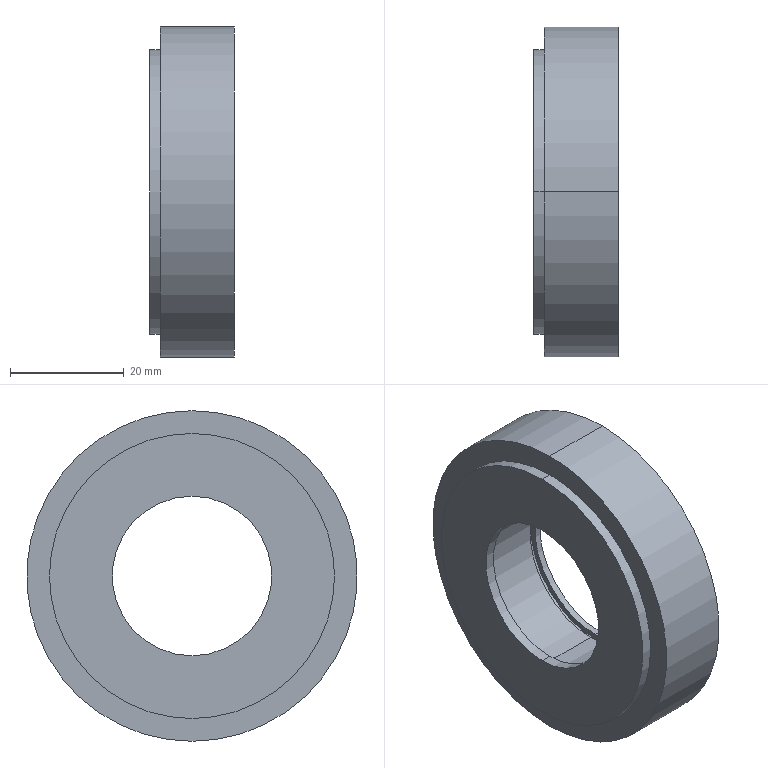Part | SolidWorks | features Revolution 1 | 1 solid | 21 faces | box 14.9 x 58 x 58 mm | volume 27501 mm3 | cylinder 14 | plane 7 | commonest cylinder face diameters 30 x4 28 x2 32 x2 34 x2 50 x2 58 x2
STEP:
#1=CARTESIAN_POINT('',(1.9,0.,25.));
#2=VERTEX_POINT('',#1);
#3=CARTESIAN_POINT('',(1.9,0.,-25.));
#4=VERTEX_POINT('',#3);
#5=CARTESIAN_POINT('',(1.9,0.,0.));
#6=DIRECTION('',(-1.,0.,0.));
#7=DIRECTION('',(0.,0.,1.));
#8=AXIS2_PLACEMENT_3D('',#5,#6,#7);
#9=CIRCLE('',#8,25.);
#10=EDGE_CURVE('',#2,#4,#9,.T.);
#11=ORIENTED_EDGE('',*,*,#10,.T.);
#12=CARTESIAN_POINT('',(0.,0.,-25.));
#13=VERTEX_POINT('',#12);
#14=CARTESIAN_POINT('',(-10.496,0.,-25.));
#15=DIRECTION('',(-1.,0.,0.));
#16=VECTOR('',#15,1000.);
#17=LINE('',#14,#16);
#18=EDGE_CURVE('',#4,#13,#17,.T.);
#19=ORIENTED_EDGE('',*,*,#18,.T.);
#20=CARTESIAN_POINT('',(0.,0.,25.));
#21=VERTEX_POINT('',#20);
#22=CARTESIAN_POINT('',(0.,0.,0.));
#23=DIRECTION('',(-1.,0.,0.));
#24=DIRECTION('',(0.,0.,1.));
#25=AXIS2_PLACEMENT_3D('',#22,#23,#24);
#26=CIRCLE('',#25,25.);
#27=EDGE_CURVE('',#21,#13,#26,.T.);
#28=ORIENTED_EDGE('',*,*,#27,.F.);
#29=CARTESIAN_POINT('',(-10.496,0.,25.));
#30=DIRECTION('',(-1.,0.,0.));
#31=VECTOR('',#30,1000.);
#32=LINE('',#29,#31);
#33=EDGE_CURVE('',#2,#21,#32,.T.);
#34=ORIENTED_EDGE('',*,*,#33,.F.);
#35=EDGE_LOOP('',(#11,#19,#28,#34));
#36=FACE_OUTER_BOUND('',#35,.T.);
#37=CARTESIAN_POINT('',(-10.496,0.,0.));
#38=DIRECTION('',(-1.,0.,0.));
#39=DIRECTION('',(0.,0.,1.));
#40=AXIS2_PLACEMENT_3D('',#37,#38,#39);
#41=CYLINDRICAL_SURFACE('',#40,25.);
#42=ADVANCED_FACE('',(#36),#41,.T.);
#43=CARTESIAN_POINT('',(14.9,0.,29.));
#44=VERTEX_POINT('',#43);
#45=CARTESIAN_POINT('',(14.9,0.,-29.));
#46=VERTEX_POINT('',#45);
#47=CARTESIAN_POINT('',(14.9,0.,0.));
#48=DIRECTION('',(-1.,0.,0.));
#49=DIRECTION('',(0.,0.,1.));
#50=AXIS2_PLACEMENT_3D('',#47,#48,#49);
#51=CIRCLE('',#50,29.);
#52=EDGE_CURVE('',#44,#46,#51,.T.);
#53=ORIENTED_EDGE('',*,*,#52,.T.);
#54=CARTESIAN_POINT('',(1.9,0.,-29.));
#55=VERTEX_POINT('',#54);
#56=CARTESIAN_POINT('',(-10.496,0.,-29.));
#57=DIRECTION('',(-1.,0.,0.));
#58=VECTOR('',#57,1000.);
#59=LINE('',#56,#58);
#60=EDGE_CURVE('',#46,#55,#59,.T.);
#61=ORIENTED_EDGE('',*,*,#60,.T.);
#62=CARTESIAN_POINT('',(1.9,0.,29.));
#63=VERTEX_POINT('',#62);
#64=CARTESIAN_POINT('',(1.9,0.,0.));
#65=DIRECTION('',(-1.,0.,0.));
#66=DIRECTION('',(0.,0.,1.));
#67=AXIS2_PLACEMENT_3D('',#64,#65,#66);
#68=CIRCLE('',#67,29.);
#69=EDGE_CURVE('',#63,#55,#68,.T.);
#70=ORIENTED_EDGE('',*,*,#69,.F.);
#71=CARTESIAN_POINT('',(-10.496,0.,29.));
#72=DIRECTION('',(-1.,0.,0.));
#73=VECTOR('',#72,1000.);
#74=LINE('',#71,#73);
#75=EDGE_CURVE('',#44,#63,#74,.T.);
#76=ORIENTED_EDGE('',*,*,#75,.F.);
#77=EDGE_LOOP('',(#53,#61,#70,#76));
#78=FACE_OUTER_BOUND('',#77,.T.);
#79=CARTESIAN_POINT('',(-10.496,0.,0.));
#80=DIRECTION('',(-1.,0.,0.));
#81=DIRECTION('',(0.,0.,1.));
#82=AXIS2_PLACEMENT_3D('',#79,#80,#81);
#83=CYLINDRICAL_SURFACE('',#82,29.);
#84=ADVANCED_FACE('',(#78),#83,.T.);
#85=CARTESIAN_POINT('',(14.9,0.,-17.));
#86=VERTEX_POINT('',#85);
#87=CARTESIAN_POINT('',(14.9,0.,17.));
#88=VERTEX_POINT('',#87);
#89=CARTESIAN_POINT('',(14.9,0.,0.));
#90=DIRECTION('',(-1.,0.,0.));
#91=DIRECTION('',(0.,0.,1.));
#92=AXIS2_PLACEMENT_3D('',#89,#90,#91);
#93=CIRCLE('',#92,17.);
#94=EDGE_CURVE('',#86,#88,#93,.T.);
#95=ORIENTED_EDGE('',*,*,#94,.F.);
#96=CARTESIAN_POINT('',(14.4,0.,-17.));
#97=VERTEX_POINT('',#96);
#98=CARTESIAN_POINT('',(-10.496,0.,-17.));
#99=DIRECTION('',(-1.,0.,0.));
#100=VECTOR('',#99,1000.);
#101=LINE('',#98,#100);
#102=EDGE_CURVE('',#86,#97,#101,.T.);
#103=ORIENTED_EDGE('',*,*,#102,.T.);
#104=CARTESIAN_POINT('',(14.4,0.,17.));
#105=VERTEX_POINT('',#104);
#106=CARTESIAN_POINT('',(14.4,0.,0.));
#107=DIRECTION('',(-1.,0.,0.));
#108=DIRECTION('',(0.,0.,1.));
#109=AXIS2_PLACEMENT_3D('',#106,#107,#108);
#110=CIRCLE('',#109,17.);
#111=EDGE_CURVE('',#97,#105,#110,.T.);
#112=ORIENTED_EDGE('',*,*,#111,.T.);
#113=CARTESIAN_POINT('',(-10.496,0.,17.));
#114=DIRECTION('',(-1.,0.,0.));
#115=VECTOR('',#114,1000.);
#116=LINE('',#113,#115);
#117=EDGE_CURVE('',#88,#105,#116,.T.);
#118=ORIENTED_EDGE('',*,*,#117,.F.);
#119=EDGE_LOOP('',(#95,#103,#112,#118));
#120=FACE_OUTER_BOUND('',#119,.T.);
#121=CARTESIAN_POINT('',(-10.496,0.,0.));
#122=DIRECTION('',(-1.,0.,0.));
#123=DIRECTION('',(0.,0.,1.));
#124=AXIS2_PLACEMENT_3D('',#121,#122,#123);
#125=CYLINDRICAL_SURFACE('',#124,17.);
#126=ADVANCED_FACE('',(#120),#125,.F.);
#127=CARTESIAN_POINT('',(14.4,0.,-15.));
#128=VERTEX_POINT('',#127);
#129=CARTESIAN_POINT('',(14.4,0.,15.));
#130=VERTEX_POINT('',#129);
#131=CARTESIAN_POINT('',(14.4,0.,0.));
#132=DIRECTION('',(-1.,0.,0.));
#133=DIRECTION('',(0.,0.,1.));
#134=AXIS2_PLACEMENT_3D('',#131,#132,#133);
#135=CIRCLE('',#134,15.);
#136=EDGE_CURVE('',#128,#130,#135,.T.);
#137=ORIENTED_EDGE('',*,*,#136,.F.);
#138=CARTESIAN_POINT('',(13.2,0.,-15.));
#139=VERTEX_POINT('',#138);
#140=CARTESIAN_POINT('',(-10.496,0.,-15.));
#141=DIRECTION('',(-1.,0.,0.));
#142=VECTOR('',#141,1000.);
#143=LINE('',#140,#142);
#144=EDGE_CURVE('',#128,#139,#143,.T.);
#145=ORIENTED_EDGE('',*,*,#144,.T.);
#146=CARTESIAN_POINT('',(13.2,0.,15.));
#147=VERTEX_POINT('',#146);
#148=CARTESIAN_POINT('',(13.2,0.,0.));
#149=DIRECTION('',(-1.,0.,0.));
#150=DIRECTION('',(0.,0.,1.));
#151=AXIS2_PLACEMENT_3D('',#148,#149,#150);
#152=CIRCLE('',#151,15.);
#153=EDGE_CURVE('',#139,#147,#152,.T.);
#154=ORIENTED_EDGE('',*,*,#153,.T.);
#155=CARTESIAN_POINT('',(-10.496,0.,15.));
#156=DIRECTION('',(-1.,0.,0.));
#157=VECTOR('',#156,1000.);
#158=LINE('',#155,#157);
#159=EDGE_CURVE('',#130,#147,#158,.T.);
#160=ORIENTED_EDGE('',*,*,#159,.F.);
#161=EDGE_LOOP('',(#137,#145,#154,#160));
#162=FACE_OUTER_BOUND('',#161,.T.);
#163=CARTESIAN_POINT('',(-10.496,0.,0.));
#164=DIRECTION('',(-1.,0.,0.));
#165=DIRECTION('',(0.,0.,1.));
#166=AXIS2_PLACEMENT_3D('',#163,#164,#165);
#167=CYLINDRICAL_SURFACE('',#166,15.);
#168=ADVANCED_FACE('',(#162),#167,.F.);
#169=CARTESIAN_POINT('',(13.2,0.,-16.));
#170=VERTEX_POINT('',#169);
#171=CARTESIAN_POINT('',(13.2,0.,16.));
#172=VERTEX_POINT('',#171);
#173=CARTESIAN_POINT('',(13.2,0.,0.));
#174=DIRECTION('',(-1.,0.,0.));
#175=DIRECTION('',(0.,0.,1.));
#176=AXIS2_PLACEMENT_3D('',#173,#174,#175);
#177=CIRCLE('',#176,16.);
#178=EDGE_CURVE('',#170,#172,#177,.T.);
#179=ORIENTED_EDGE('',*,*,#178,.F.);
#180=CARTESIAN_POINT('',(12.,0.,-16.));
#181=VERTEX_POINT('',#180);
#182=CARTESIAN_POINT('',(-10.496,0.,-16.));
#183=DIRECTION('',(-1.,0.,0.));
#184=VECTOR('',#183,1000.);
#185=LINE('',#182,#184);
#186=EDGE_CURVE('',#170,#181,#185,.T.);
#187=ORIENTED_EDGE('',*,*,#186,.T.);
#188=CARTESIAN_POINT('',(12.,0.,16.));
#189=VERTEX_POINT('',#188);
#190=CARTESIAN_POINT('',(12.,0.,0.));
#191=DIRECTION('',(-1.,0.,0.));
#192=DIRECTION('',(0.,0.,1.));
#193=AXIS2_PLACEMENT_3D('',#190,#191,#192);
#194=CIRCLE('',#193,16.);
#195=EDGE_CURVE('',#181,#189,#194,.T.);
#196=ORIENTED_EDGE('',*,*,#195,.T.);
#197=CARTESIAN_POINT('',(-10.496,0.,16.));
#198=DIRECTION('',(-1.,0.,0.));
#199=VECTOR('',#198,1000.);
#200=LINE('',#197,#199);
#201=EDGE_CURVE('',#172,#189,#200,.T.);
#202=ORIENTED_EDGE('',*,*,#201,.F.);
#203=EDGE_LOOP('',(#179,#187,#196,#202));
#204=FACE_OUTER_BOUND('',#203,.T.);
#205=CARTESIAN_POINT('',(-10.496,0.,0.));
#206=DIRECTION('',(-1.,0.,0.));
#207=DIRECTION('',(0.,0.,1.));
#208=AXIS2_PLACEMENT_3D('',#205,#206,#207);
#209=CYLINDRICAL_SURFACE('',#208,16.);
#210=ADVANCED_FACE('',(#204),#209,.F.);
#211=CARTESIAN_POINT('',(12.,0.,-15.));
#212=VERTEX_POINT('',#211);
#213=CARTESIAN_POINT('',(12.,0.,15.));
#214=VERTEX_POINT('',#213);
#215=CARTESIAN_POINT('',(12.,0.,0.));
#216=DIRECTION('',(-1.,0.,0.));
#217=DIRECTION('',(0.,0.,1.));
#218=AXIS2_PLACEMENT_3D('',#215,#216,#217);
#219=CIRCLE('',#218,15.);
#220=EDGE_CURVE('',#212,#214,#219,.T.);
#221=ORIENTED_EDGE('',*,*,#220,.F.);
#222=CARTESIAN_POINT('',(1.9,0.,-15.));
#223=VERTEX_POINT('',#222);
#224=CARTESIAN_POINT('',(-10.496,0.,-15.));
#225=DIRECTION('',(-1.,0.,0.));
#226=VECTOR('',#225,1000.);
#227=LINE('',#224,#226);
#228=EDGE_CURVE('',#212,#223,#227,.T.);
#229=ORIENTED_EDGE('',*,*,#228,.T.);
#230=CARTESIAN_POINT('',(1.9,0.,15.));
#231=VERTEX_POINT('',#230);
#232=CARTESIAN_POINT('',(1.9,0.,0.));
#233=DIRECTION('',(-1.,0.,0.));
#234=DIRECTION('',(0.,0.,1.));
#235=AXIS2_PLACEMENT_3D('',#232,#233,#234);
#236=CIRCLE('',#235,15.);
#237=EDGE_CURVE('',#223,#231,#236,.T.);
#238=ORIENTED_EDGE('',*,*,#237,.T.);
#239=CARTESIAN_POINT('',(-10.496,0.,15.));
#240=DIRECTION('',(-1.,0.,0.));
#241=VECTOR('',#240,1000.);
#242=LINE('',#239,#241);
#243=EDGE_CURVE('',#214,#231,#242,.T.);
#244=ORIENTED_EDGE('',*,*,#243,.F.);
#245=EDGE_LOOP('',(#221,#229,#238,#244));
#246=FACE_OUTER_BOUND('',#245,.T.);
#247=CARTESIAN_POINT('',(-10.496,0.,0.));
#248=DIRECTION('',(-1.,0.,0.));
#249=DIRECTION('',(0.,0.,1.));
#250=AXIS2_PLACEMENT_3D('',#247,#248,#249);
#251=CYLINDRICAL_SURFACE('',#250,15.);
#252=ADVANCED_FACE('',(#246),#251,.F.);
#253=CARTESIAN_POINT('',(1.9,0.,-14.));
#254=VERTEX_POINT('',#253);
#255=CARTESIAN_POINT('',(1.9,0.,14.));
#256=VERTEX_POINT('',#255);
#257=CARTESIAN_POINT('',(1.9,0.,0.));
#258=DIRECTION('',(-1.,0.,0.));
#259=DIRECTION('',(0.,0.,1.));
#260=AXIS2_PLACEMENT_3D('',#257,#258,#259);
#261=CIRCLE('',#260,14.);
#262=EDGE_CURVE('',#254,#256,#261,.T.);
#263=ORIENTED_EDGE('',*,*,#262,.F.);
#264=CARTESIAN_POINT('',(0.,0.,-14.));
#265=VERTEX_POINT('',#264);
#266=CARTESIAN_POINT('',(-10.496,0.,-14.));
#267=DIRECTION('',(-1.,0.,0.));
#268=VECTOR('',#267,1000.);
#269=LINE('',#266,#268);
#270=EDGE_CURVE('',#254,#265,#269,.T.);
#271=ORIENTED_EDGE('',*,*,#270,.T.);
#272=CARTESIAN_POINT('',(0.,0.,14.));
#273=VERTEX_POINT('',#272);
#274=CARTESIAN_POINT('',(0.,0.,0.));
#275=DIRECTION('',(-1.,0.,0.));
#276=DIRECTION('',(0.,0.,1.));
#277=AXIS2_PLACEMENT_3D('',#274,#275,#276);
#278=CIRCLE('',#277,14.);
#279=EDGE_CURVE('',#265,#273,#278,.T.);
#280=ORIENTED_EDGE('',*,*,#279,.T.);
#281=CARTESIAN_POINT('',(-10.496,0.,14.));
#282=DIRECTION('',(-1.,0.,0.));
#283=VECTOR('',#282,1000.);
#284=LINE('',#281,#283);
#285=EDGE_CURVE('',#256,#273,#284,.T.);
#286=ORIENTED_EDGE('',*,*,#285,.F.);
#287=EDGE_LOOP('',(#263,#271,#280,#286));
#288=FACE_OUTER_BOUND('',#287,.T.);
#289=CARTESIAN_POINT('',(-10.496,0.,0.));
#290=DIRECTION('',(-1.,0.,0.));
#291=DIRECTION('',(0.,0.,1.));
#292=AXIS2_PLACEMENT_3D('',#289,#290,#291);
#293=CYLINDRICAL_SURFACE('',#292,14.);
#294=ADVANCED_FACE('',(#288),#293,.F.);
#295=CARTESIAN_POINT('',(0.,0.,0.));
#296=DIRECTION('',(-1.,0.,0.));
#297=DIRECTION('',(0.,0.,1.));
#298=AXIS2_PLACEMENT_3D('',#295,#296,#297);
#299=CIRCLE('',#298,14.);
#300=EDGE_CURVE('',#273,#265,#299,.T.);
#301=ORIENTED_EDGE('',*,*,#300,.F.);
#302=ORIENTED_EDGE('',*,*,#279,.F.);
#303=EDGE_LOOP('',(#301,#302));
#304=FACE_BOUND('',#303,.T.);
#305=ORIENTED_EDGE('',*,*,#27,.T.);
#306=CARTESIAN_POINT('',(0.,0.,0.));
#307=DIRECTION('',(-1.,0.,0.));
#308=DIRECTION('',(0.,0.,1.));
#309=AXIS2_PLACEMENT_3D('',#306,#307,#308);
#310=CIRCLE('',#309,25.);
#311=EDGE_CURVE('',#13,#21,#310,.T.);
#312=ORIENTED_EDGE('',*,*,#311,.T.);
#313=EDGE_LOOP('',(#305,#312));
#314=FACE_OUTER_BOUND('',#313,.T.);
#315=CARTESIAN_POINT('',(0.,25.,0.));
#316=DIRECTION('',(1.,0.,0.));
#317=DIRECTION('',(0.,0.,-1.));
#318=AXIS2_PLACEMENT_3D('',#315,#316,#317);
#319=PLANE('',#318);
#320=ADVANCED_FACE('',(#304,#314),#319,.F.);
#321=ORIENTED_EDGE('',*,*,#270,.F.);
#322=CARTESIAN_POINT('',(1.9,0.,0.));
#323=DIRECTION('',(-1.,0.,0.));
#324=DIRECTION('',(0.,0.,1.));
#325=AXIS2_PLACEMENT_3D('',#322,#323,#324);
#326=CIRCLE('',#325,14.);
#327=EDGE_CURVE('',#256,#254,#326,.T.);
#328=ORIENTED_EDGE('',*,*,#327,.F.);
#329=ORIENTED_EDGE('',*,*,#285,.T.);
#330=ORIENTED_EDGE('',*,*,#300,.T.);
#331=EDGE_LOOP('',(#321,#328,#329,#330));
#332=FACE_OUTER_BOUND('',#331,.T.);
#333=CARTESIAN_POINT('',(-10.496,0.,0.));
#334=DIRECTION('',(-1.,0.,0.));
#335=DIRECTION('',(0.,0.,1.));
#336=AXIS2_PLACEMENT_3D('',#333,#334,#335);
#337=CYLINDRICAL_SURFACE('',#336,14.);
#338=ADVANCED_FACE('',(#332),#337,.F.);
#339=CARTESIAN_POINT('',(1.9,0.,0.));
#340=DIRECTION('',(-1.,0.,0.));
#341=DIRECTION('',(0.,0.,1.));
#342=AXIS2_PLACEMENT_3D('',#339,#340,#341);
#343=CIRCLE('',#342,15.);
#344=EDGE_CURVE('',#231,#223,#343,.T.);
#345=ORIENTED_EDGE('',*,*,#344,.F.);
#346=ORIENTED_EDGE('',*,*,#237,.F.);
#347=EDGE_LOOP('',(#345,#346));
#348=FACE_OUTER_BOUND('',#347,.T.);
#349=ORIENTED_EDGE('',*,*,#327,.T.);
#350=ORIENTED_EDGE('',*,*,#262,.T.);
#351=EDGE_LOOP('',(#349,#350));
#352=FACE_BOUND('',#351,.T.);
#353=CARTESIAN_POINT('',(1.9,14.,0.));
#354=DIRECTION('',(-1.,0.,0.));
#355=DIRECTION('',(0.,0.,1.));
#356=AXIS2_PLACEMENT_3D('',#353,#354,#355);
#357=PLANE('',#356);
#358=ADVANCED_FACE('',(#348,#352),#357,.F.);
#359=ORIENTED_EDGE('',*,*,#228,.F.);
#360=CARTESIAN_POINT('',(12.,0.,0.));
#361=DIRECTION('',(-1.,0.,0.));
#362=DIRECTION('',(0.,0.,1.));
#363=AXIS2_PLACEMENT_3D('',#360,#361,#362);
#364=CIRCLE('',#363,15.);
#365=EDGE_CURVE('',#214,#212,#364,.T.);
#366=ORIENTED_EDGE('',*,*,#365,.F.);
#367=ORIENTED_EDGE('',*,*,#243,.T.);
#368=ORIENTED_EDGE('',*,*,#344,.T.);
#369=EDGE_LOOP('',(#359,#366,#367,#368));
#370=FACE_OUTER_BOUND('',#369,.T.);
#371=CARTESIAN_POINT('',(-10.496,0.,0.));
#372=DIRECTION('',(-1.,0.,0.));
#373=DIRECTION('',(0.,0.,1.));
#374=AXIS2_PLACEMENT_3D('',#371,#372,#373);
#375=CYLINDRICAL_SURFACE('',#374,15.);
#376=ADVANCED_FACE('',(#370),#375,.F.);
#377=CARTESIAN_POINT('',(12.,0.,0.));
#378=DIRECTION('',(-1.,0.,0.));
#379=DIRECTION('',(0.,0.,1.));
#380=AXIS2_PLACEMENT_3D('',#377,#378,#379);
#381=CIRCLE('',#380,16.);
#382=EDGE_CURVE('',#189,#181,#381,.T.);
#383=ORIENTED_EDGE('',*,*,#382,.F.);
#384=ORIENTED_EDGE('',*,*,#195,.F.);
#385=EDGE_LOOP('',(#383,#384));
#386=FACE_OUTER_BOUND('',#385,.T.);
#387=ORIENTED_EDGE('',*,*,#365,.T.);
#388=ORIENTED_EDGE('',*,*,#220,.T.);
#389=EDGE_LOOP('',(#387,#388));
#390=FACE_BOUND('',#389,.T.);
#391=CARTESIAN_POINT('',(12.,15.,0.));
#392=DIRECTION('',(-1.,0.,0.));
#393=DIRECTION('',(0.,0.,1.));
#394=AXIS2_PLACEMENT_3D('',#391,#392,#393);
#395=PLANE('',#394);
#396=ADVANCED_FACE('',(#386,#390),#395,.F.);
#397=ORIENTED_EDGE('',*,*,#186,.F.);
#398=CARTESIAN_POINT('',(13.2,0.,0.));
#399=DIRECTION('',(-1.,0.,0.));
#400=DIRECTION('',(0.,0.,1.));
#401=AXIS2_PLACEMENT_3D('',#398,#399,#400);
#402=CIRCLE('',#401,16.);
#403=EDGE_CURVE('',#172,#170,#402,.T.);
#404=ORIENTED_EDGE('',*,*,#403,.F.);
#405=ORIENTED_EDGE('',*,*,#201,.T.);
#406=ORIENTED_EDGE('',*,*,#382,.T.);
#407=EDGE_LOOP('',(#397,#404,#405,#406));
#408=FACE_OUTER_BOUND('',#407,.T.);
#409=CARTESIAN_POINT('',(-10.496,0.,0.));
#410=DIRECTION('',(-1.,0.,0.));
#411=DIRECTION('',(0.,0.,1.));
#412=AXIS2_PLACEMENT_3D('',#409,#410,#411);
#413=CYLINDRICAL_SURFACE('',#412,16.);
#414=ADVANCED_FACE('',(#408),#413,.F.);
#415=CARTESIAN_POINT('',(13.2,0.,0.));
#416=DIRECTION('',(-1.,0.,0.));
#417=DIRECTION('',(0.,0.,1.));
#418=AXIS2_PLACEMENT_3D('',#415,#416,#417);
#419=CIRCLE('',#418,15.);
#420=EDGE_CURVE('',#147,#139,#419,.T.);
#421=ORIENTED_EDGE('',*,*,#420,.F.);
#422=ORIENTED_EDGE('',*,*,#153,.F.);
#423=EDGE_LOOP('',(#421,#422));
#424=FACE_BOUND('',#423,.T.);
#425=ORIENTED_EDGE('',*,*,#403,.T.);
#426=ORIENTED_EDGE('',*,*,#178,.T.);
#427=EDGE_LOOP('',(#425,#426));
#428=FACE_OUTER_BOUND('',#427,.T.);
#429=CARTESIAN_POINT('',(13.2,16.,0.));
#430=DIRECTION('',(1.,0.,0.));
#431=DIRECTION('',(0.,0.,-1.));
#432=AXIS2_PLACEMENT_3D('',#429,#430,#431);
#433=PLANE('',#432);
#434=ADVANCED_FACE('',(#424,#428),#433,.F.);
#435=ORIENTED_EDGE('',*,*,#144,.F.);
#436=CARTESIAN_POINT('',(14.4,0.,0.));
#437=DIRECTION('',(-1.,0.,0.));
#438=DIRECTION('',(0.,0.,1.));
#439=AXIS2_PLACEMENT_3D('',#436,#437,#438);
#440=CIRCLE('',#439,15.);
#441=EDGE_CURVE('',#130,#128,#440,.T.);
#442=ORIENTED_EDGE('',*,*,#441,.F.);
#443=ORIENTED_EDGE('',*,*,#159,.T.);
#444=ORIENTED_EDGE('',*,*,#420,.T.);
#445=EDGE_LOOP('',(#435,#442,#443,#444));
#446=FACE_OUTER_BOUND('',#445,.T.);
#447=CARTESIAN_POINT('',(-10.496,0.,0.));
#448=DIRECTION('',(-1.,0.,0.));
#449=DIRECTION('',(0.,0.,1.));
#450=AXIS2_PLACEMENT_3D('',#447,#448,#449);
#451=CYLINDRICAL_SURFACE('',#450,15.);
#452=ADVANCED_FACE('',(#446),#451,.F.);
#453=CARTESIAN_POINT('',(14.4,0.,0.));
#454=DIRECTION('',(-1.,0.,0.));
#455=DIRECTION('',(0.,0.,1.));
#456=AXIS2_PLACEMENT_3D('',#453,#454,#455);
#457=CIRCLE('',#456,17.);
#458=EDGE_CURVE('',#105,#97,#457,.T.);
#459=ORIENTED_EDGE('',*,*,#458,.F.);
#460=ORIENTED_EDGE('',*,*,#111,.F.);
#461=EDGE_LOOP('',(#459,#460));
#462=FACE_OUTER_BOUND('',#461,.T.);
#463=ORIENTED_EDGE('',*,*,#441,.T.);
#464=ORIENTED_EDGE('',*,*,#136,.T.);
#465=EDGE_LOOP('',(#463,#464));
#466=FACE_BOUND('',#465,.T.);
#467=CARTESIAN_POINT('',(14.4,15.,0.));
#468=DIRECTION('',(-1.,0.,0.));
#469=DIRECTION('',(0.,0.,1.));
#470=AXIS2_PLACEMENT_3D('',#467,#468,#469);
#471=PLANE('',#470);
#472=ADVANCED_FACE('',(#462,#466),#471,.F.);
#473=ORIENTED_EDGE('',*,*,#102,.F.);
#474=CARTESIAN_POINT('',(14.9,0.,0.));
#475=DIRECTION('',(-1.,0.,0.));
#476=DIRECTION('',(0.,0.,1.));
#477=AXIS2_PLACEMENT_3D('',#474,#475,#476);
#478=CIRCLE('',#477,17.);
#479=EDGE_CURVE('',#88,#86,#478,.T.);
#480=ORIENTED_EDGE('',*,*,#479,.F.);
#481=ORIENTED_EDGE('',*,*,#117,.T.);
#482=ORIENTED_EDGE('',*,*,#458,.T.);
#483=EDGE_LOOP('',(#473,#480,#481,#482));
#484=FACE_OUTER_BOUND('',#483,.T.);
#485=CARTESIAN_POINT('',(-10.496,0.,0.));
#486=DIRECTION('',(-1.,0.,0.));
#487=DIRECTION('',(0.,0.,1.));
#488=AXIS2_PLACEMENT_3D('',#485,#486,#487);
#489=CYLINDRICAL_SURFACE('',#488,17.);
#490=ADVANCED_FACE('',(#484),#489,.F.);
#491=ORIENTED_EDGE('',*,*,#52,.F.);
#492=CARTESIAN_POINT('',(14.9,0.,0.));
#493=DIRECTION('',(-1.,0.,0.));
#494=DIRECTION('',(0.,0.,1.));
#495=AXIS2_PLACEMENT_3D('',#492,#493,#494);
#496=CIRCLE('',#495,29.);
#497=EDGE_CURVE('',#46,#44,#496,.T.);
#498=ORIENTED_EDGE('',*,*,#497,.F.);
#499=EDGE_LOOP('',(#491,#498));
#500=FACE_OUTER_BOUND('',#499,.T.);
#501=ORIENTED_EDGE('',*,*,#479,.T.);
#502=ORIENTED_EDGE('',*,*,#94,.T.);
#503=EDGE_LOOP('',(#501,#502));
#504=FACE_BOUND('',#503,.T.);
#505=CARTESIAN_POINT('',(14.9,17.,0.));
#506=DIRECTION('',(-1.,0.,0.));
#507=DIRECTION('',(0.,0.,1.));
#508=AXIS2_PLACEMENT_3D('',#505,#506,#507);
#509=PLANE('',#508);
#510=ADVANCED_FACE('',(#500,#504),#509,.F.);
#511=ORIENTED_EDGE('',*,*,#60,.F.);
#512=ORIENTED_EDGE('',*,*,#497,.T.);
#513=ORIENTED_EDGE('',*,*,#75,.T.);
#514=CARTESIAN_POINT('',(1.9,0.,0.));
#515=DIRECTION('',(-1.,0.,0.));
#516=DIRECTION('',(0.,0.,1.));
#517=AXIS2_PLACEMENT_3D('',#514,#515,#516);
#518=CIRCLE('',#517,29.);
#519=EDGE_CURVE('',#55,#63,#518,.T.);
#520=ORIENTED_EDGE('',*,*,#519,.F.);
#521=EDGE_LOOP('',(#511,#512,#513,#520));
#522=FACE_OUTER_BOUND('',#521,.T.);
#523=CARTESIAN_POINT('',(-10.496,0.,0.));
#524=DIRECTION('',(-1.,0.,0.));
#525=DIRECTION('',(0.,0.,1.));
#526=AXIS2_PLACEMENT_3D('',#523,#524,#525);
#527=CYLINDRICAL_SURFACE('',#526,29.);
#528=ADVANCED_FACE('',(#522),#527,.T.);
#529=ORIENTED_EDGE('',*,*,#10,.F.);
#530=CARTESIAN_POINT('',(1.9,0.,0.));
#531=DIRECTION('',(-1.,0.,0.));
#532=DIRECTION('',(0.,0.,1.));
#533=AXIS2_PLACEMENT_3D('',#530,#531,#532);
#534=CIRCLE('',#533,25.);
#535=EDGE_CURVE('',#4,#2,#534,.T.);
#536=ORIENTED_EDGE('',*,*,#535,.F.);
#537=EDGE_LOOP('',(#529,#536));
#538=FACE_BOUND('',#537,.T.);
#539=ORIENTED_EDGE('',*,*,#69,.T.);
#540=ORIENTED_EDGE('',*,*,#519,.T.);
#541=EDGE_LOOP('',(#539,#540));
#542=FACE_OUTER_BOUND('',#541,.T.);
#543=CARTESIAN_POINT('',(1.9,29.,0.));
#544=DIRECTION('',(1.,0.,0.));
#545=DIRECTION('',(0.,0.,-1.));
#546=AXIS2_PLACEMENT_3D('',#543,#544,#545);
#547=PLANE('',#546);
#548=ADVANCED_FACE('',(#538,#542),#547,.F.);
#549=ORIENTED_EDGE('',*,*,#18,.F.);
#550=ORIENTED_EDGE('',*,*,#535,.T.);
#551=ORIENTED_EDGE('',*,*,#33,.T.);
#552=ORIENTED_EDGE('',*,*,#311,.F.);
#553=EDGE_LOOP('',(#549,#550,#551,#552));
#554=FACE_OUTER_BOUND('',#553,.T.);
#555=CARTESIAN_POINT('',(-10.496,0.,0.));
#556=DIRECTION('',(-1.,0.,0.));
#557=DIRECTION('',(0.,0.,1.));
#558=AXIS2_PLACEMENT_3D('',#555,#556,#557);
#559=CYLINDRICAL_SURFACE('',#558,25.);
#560=ADVANCED_FACE('',(#554),#559,.T.);
#561=CLOSED_SHELL('',(#42,#84,#126,#168,#210,#252,#294,#320,#338,#358,#376,#396,#414,#434,#452,#472,#490,#510,#528,#548,#560));
#562=MANIFOLD_SOLID_BREP('',#561);
#563=CARTESIAN_POINT('',(0.,0.,0.));
#564=DIRECTION('',(0.,0.,1.));
#565=DIRECTION('',(1.,0.,0.));
#566=AXIS2_PLACEMENT_3D('',#563,#564,#565);
#567=(LENGTH_UNIT()NAMED_UNIT(*)SI_UNIT(.MILLI.,.METRE.));
#568=UNCERTAINTY_MEASURE_WITH_UNIT(LENGTH_MEASURE(0.00001),#567,'','');
#569=(NAMED_UNIT(*)PLANE_ANGLE_UNIT()SI_UNIT($,.RADIAN.));
#570=(NAMED_UNIT(*)SI_UNIT($,.STERADIAN.)SOLID_ANGLE_UNIT());
#571=(GEOMETRIC_REPRESENTATION_CONTEXT(3)GLOBAL_UNCERTAINTY_ASSIGNED_CONTEXT((#568))GLOBAL_UNIT_ASSIGNED_CONTEXT((#567,#569,#570))REPRESENTATION_CONTEXT('',''));
#572=ADVANCED_BREP_SHAPE_REPRESENTATION('',(#562,#566),#571);